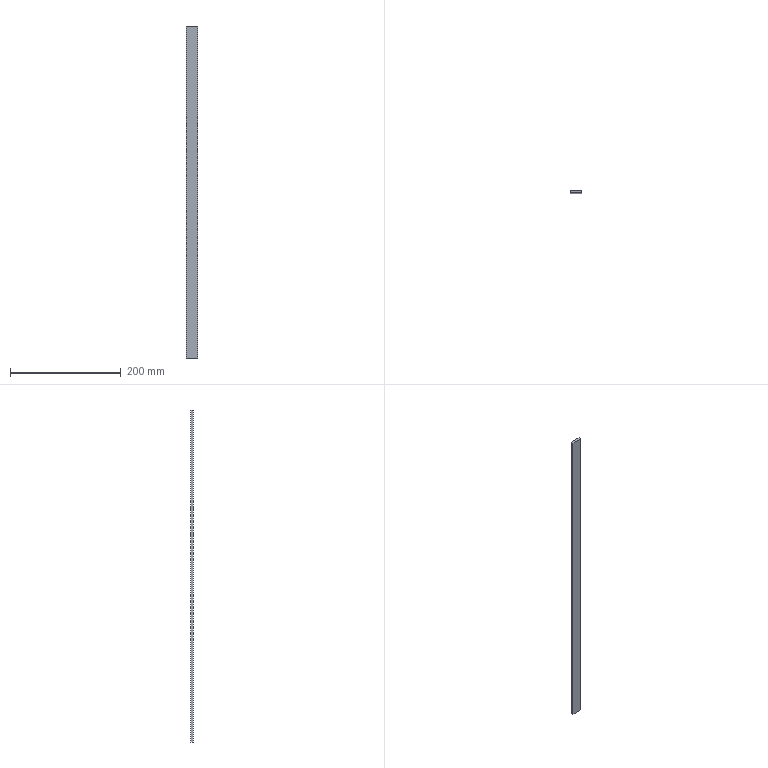Part | STEP file | Guide wheel mechanism revised.sldasm-Part-87 | 1 solid | 6 faces | box 20 x 4.5 x 600 mm | volume 54000 mm3 | plane 6
STEP:
#1=CARTESIAN_POINT('',(-10.,21.95,-600.));
#2=VERTEX_POINT('',#1);
#3=CARTESIAN_POINT('',(-10.,26.45,-600.));
#4=VERTEX_POINT('',#3);
#5=CARTESIAN_POINT('',(-10.,26.45,-600.));
#6=DIRECTION('',(0.,1.,0.));
#7=VECTOR('',#6,1000.);
#8=LINE('',#5,#7);
#9=EDGE_CURVE('',#2,#4,#8,.T.);
#10=ORIENTED_EDGE('',*,*,#9,.F.);
#11=CARTESIAN_POINT('',(-10.,21.95,0.));
#12=VERTEX_POINT('',#11);
#13=CARTESIAN_POINT('',(-10.,21.95,-620.57));
#14=DIRECTION('',(0.,0.,1.));
#15=VECTOR('',#14,1000.);
#16=LINE('',#13,#15);
#17=EDGE_CURVE('',#2,#12,#16,.T.);
#18=ORIENTED_EDGE('',*,*,#17,.T.);
#19=CARTESIAN_POINT('',(-10.,26.45,0.));
#20=VERTEX_POINT('',#19);
#21=CARTESIAN_POINT('',(-10.,26.45,0.));
#22=DIRECTION('',(0.,-1.,0.));
#23=VECTOR('',#22,1000.);
#24=LINE('',#21,#23);
#25=EDGE_CURVE('',#20,#12,#24,.T.);
#26=ORIENTED_EDGE('',*,*,#25,.F.);
#27=CARTESIAN_POINT('',(-10.,26.45,-620.57));
#28=DIRECTION('',(0.,0.,1.));
#29=VECTOR('',#28,1000.);
#30=LINE('',#27,#29);
#31=EDGE_CURVE('',#4,#20,#30,.T.);
#32=ORIENTED_EDGE('',*,*,#31,.F.);
#33=EDGE_LOOP('',(#10,#18,#26,#32));
#34=FACE_OUTER_BOUND('',#33,.T.);
#35=CARTESIAN_POINT('',(-10.,26.45,-620.57));
#36=DIRECTION('',(-1.,0.,0.));
#37=DIRECTION('',(0.,-1.,0.));
#38=AXIS2_PLACEMENT_3D('',#35,#36,#37);
#39=PLANE('',#38);
#40=ADVANCED_FACE('',(#34),#39,.T.);
#41=CARTESIAN_POINT('',(10.,26.45,-600.));
#42=VERTEX_POINT('',#41);
#43=CARTESIAN_POINT('',(-10.,26.45,-600.));
#44=DIRECTION('',(1.,0.,0.));
#45=VECTOR('',#44,1000.);
#46=LINE('',#43,#45);
#47=EDGE_CURVE('',#4,#42,#46,.T.);
#48=ORIENTED_EDGE('',*,*,#47,.F.);
#49=ORIENTED_EDGE('',*,*,#31,.T.);
#50=CARTESIAN_POINT('',(10.,26.45,0.));
#51=VERTEX_POINT('',#50);
#52=CARTESIAN_POINT('',(-10.,26.45,0.));
#53=DIRECTION('',(-1.,0.,0.));
#54=VECTOR('',#53,1000.);
#55=LINE('',#52,#54);
#56=EDGE_CURVE('',#51,#20,#55,.T.);
#57=ORIENTED_EDGE('',*,*,#56,.F.);
#58=CARTESIAN_POINT('',(10.,26.45,-620.57));
#59=DIRECTION('',(0.,0.,1.));
#60=VECTOR('',#59,1000.);
#61=LINE('',#58,#60);
#62=EDGE_CURVE('',#42,#51,#61,.T.);
#63=ORIENTED_EDGE('',*,*,#62,.F.);
#64=EDGE_LOOP('',(#48,#49,#57,#63));
#65=FACE_OUTER_BOUND('',#64,.T.);
#66=CARTESIAN_POINT('',(-10.,26.45,-620.57));
#67=DIRECTION('',(0.,1.,0.));
#68=DIRECTION('',(0.,0.,1.));
#69=AXIS2_PLACEMENT_3D('',#66,#67,#68);
#70=PLANE('',#69);
#71=ADVANCED_FACE('',(#65),#70,.T.);
#72=CARTESIAN_POINT('',(10.,21.95,-600.));
#73=VERTEX_POINT('',#72);
#74=CARTESIAN_POINT('',(10.,26.45,-600.));
#75=DIRECTION('',(0.,-1.,0.));
#76=VECTOR('',#75,1000.);
#77=LINE('',#74,#76);
#78=EDGE_CURVE('',#42,#73,#77,.T.);
#79=ORIENTED_EDGE('',*,*,#78,.F.);
#80=ORIENTED_EDGE('',*,*,#62,.T.);
#81=CARTESIAN_POINT('',(10.,21.95,0.));
#82=VERTEX_POINT('',#81);
#83=CARTESIAN_POINT('',(10.,26.45,0.));
#84=DIRECTION('',(0.,1.,0.));
#85=VECTOR('',#84,1000.);
#86=LINE('',#83,#85);
#87=EDGE_CURVE('',#82,#51,#86,.T.);
#88=ORIENTED_EDGE('',*,*,#87,.F.);
#89=CARTESIAN_POINT('',(10.,21.95,-620.57));
#90=DIRECTION('',(0.,0.,1.));
#91=VECTOR('',#90,1000.);
#92=LINE('',#89,#91);
#93=EDGE_CURVE('',#73,#82,#92,.T.);
#94=ORIENTED_EDGE('',*,*,#93,.F.);
#95=EDGE_LOOP('',(#79,#80,#88,#94));
#96=FACE_OUTER_BOUND('',#95,.T.);
#97=CARTESIAN_POINT('',(10.,26.45,-620.57));
#98=DIRECTION('',(1.,0.,0.));
#99=DIRECTION('',(0.,1.,0.));
#100=AXIS2_PLACEMENT_3D('',#97,#98,#99);
#101=PLANE('',#100);
#102=ADVANCED_FACE('',(#96),#101,.T.);
#103=CARTESIAN_POINT('',(-10.,21.95,-600.));
#104=DIRECTION('',(-1.,0.,0.));
#105=VECTOR('',#104,1000.);
#106=LINE('',#103,#105);
#107=EDGE_CURVE('',#73,#2,#106,.T.);
#108=ORIENTED_EDGE('',*,*,#107,.F.);
#109=ORIENTED_EDGE('',*,*,#93,.T.);
#110=CARTESIAN_POINT('',(-10.,21.95,0.));
#111=DIRECTION('',(1.,0.,0.));
#112=VECTOR('',#111,1000.);
#113=LINE('',#110,#112);
#114=EDGE_CURVE('',#12,#82,#113,.T.);
#115=ORIENTED_EDGE('',*,*,#114,.F.);
#116=ORIENTED_EDGE('',*,*,#17,.F.);
#117=EDGE_LOOP('',(#108,#109,#115,#116));
#118=FACE_OUTER_BOUND('',#117,.T.);
#119=CARTESIAN_POINT('',(-10.,21.95,-620.57));
#120=DIRECTION('',(0.,-1.,0.));
#121=DIRECTION('',(0.,0.,-1.));
#122=AXIS2_PLACEMENT_3D('',#119,#120,#121);
#123=PLANE('',#122);
#124=ADVANCED_FACE('',(#118),#123,.T.);
#125=ORIENTED_EDGE('',*,*,#25,.T.);
#126=ORIENTED_EDGE('',*,*,#114,.T.);
#127=ORIENTED_EDGE('',*,*,#87,.T.);
#128=ORIENTED_EDGE('',*,*,#56,.T.);
#129=EDGE_LOOP('',(#125,#126,#127,#128));
#130=FACE_OUTER_BOUND('',#129,.T.);
#131=CARTESIAN_POINT('',(0.,0.,0.));
#132=DIRECTION('',(0.,0.,1.));
#133=DIRECTION('',(1.,0.,0.));
#134=AXIS2_PLACEMENT_3D('',#131,#132,#133);
#135=PLANE('',#134);
#136=ADVANCED_FACE('',(#130),#135,.T.);
#137=ORIENTED_EDGE('',*,*,#9,.T.);
#138=ORIENTED_EDGE('',*,*,#47,.T.);
#139=ORIENTED_EDGE('',*,*,#78,.T.);
#140=ORIENTED_EDGE('',*,*,#107,.T.);
#141=EDGE_LOOP('',(#137,#138,#139,#140));
#142=FACE_OUTER_BOUND('',#141,.T.);
#143=CARTESIAN_POINT('',(-14.837,-23.55,-600.));
#144=DIRECTION('',(0.,0.,1.));
#145=DIRECTION('',(1.,0.,0.));
#146=AXIS2_PLACEMENT_3D('',#143,#144,#145);
#147=PLANE('',#146);
#148=ADVANCED_FACE('',(#142),#147,.F.);
#149=CLOSED_SHELL('',(#40,#71,#102,#124,#136,#148));
#150=MANIFOLD_SOLID_BREP('',#149);
#151=CARTESIAN_POINT('',(0.,0.,0.));
#152=DIRECTION('',(0.,0.,1.));
#153=DIRECTION('',(1.,0.,0.));
#154=AXIS2_PLACEMENT_3D('',#151,#152,#153);
#155=(LENGTH_UNIT()NAMED_UNIT(*)SI_UNIT(.MILLI.,.METRE.));
#156=UNCERTAINTY_MEASURE_WITH_UNIT(LENGTH_MEASURE(0.00001),#155,'','');
#157=(NAMED_UNIT(*)PLANE_ANGLE_UNIT()SI_UNIT($,.RADIAN.));
#158=(NAMED_UNIT(*)SI_UNIT($,.STERADIAN.)SOLID_ANGLE_UNIT());
#159=(GEOMETRIC_REPRESENTATION_CONTEXT(3)GLOBAL_UNCERTAINTY_ASSIGNED_CONTEXT((#156))GLOBAL_UNIT_ASSIGNED_CONTEXT((#155,#157,#158))REPRESENTATION_CONTEXT('',''));
#160=ADVANCED_BREP_SHAPE_REPRESENTATION('',(#150,#154),#159);